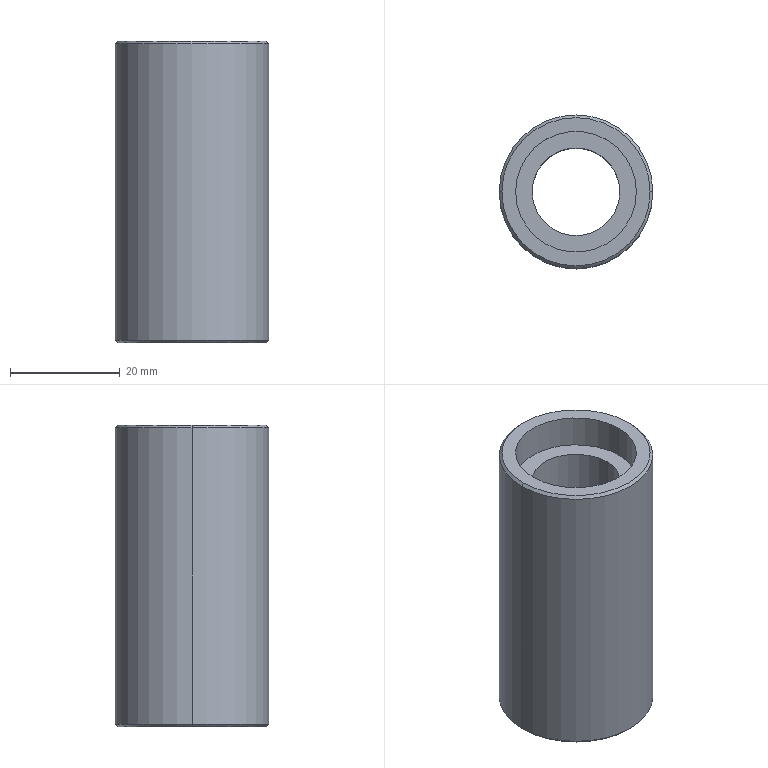Part | STEP file | 2017 Hold-down shaft | 1 solid | 16 faces | box 28 x 28 x 55 mm | volume 20637 mm3 | cylinder 8 | cone 4 | plane 4 | commonest cylinder face diameters 22 x4 16 x2 28 x2
STEP:
#1=CARTESIAN_POINT('',(0.,0.,0.));
#2=DIRECTION('',(0.,0.,1.));
#3=DIRECTION('',(1.,0.,0.));
#4=AXIS2_PLACEMENT_3D('',#1,#2,#3);
#5=CARTESIAN_POINT('',(-11.,0.,6.));
#6=VERTEX_POINT('',#5);
#7=CARTESIAN_POINT('',(-11.,0.,0.));
#8=VERTEX_POINT('',#7);
#9=CARTESIAN_POINT('',(-11.,0.,6.));
#10=DIRECTION('',(0.,0.,-1.));
#11=VECTOR('',#10,1.);
#12=LINE('',#9,#11);
#13=CARTESIAN_POINT('',(0.,0.,6.));
#14=DIRECTION('',(0.,0.,-1.));
#15=DIRECTION('',(-1.,0.,0.));
#16=AXIS2_PLACEMENT_3D('',#13,#14,#15);
#17=CYLINDRICAL_SURFACE('',#16,11.);
#18=CARTESIAN_POINT('',(6.283,0.));
#19=DIRECTION('',(0.,1.));
#20=VECTOR('',#19,1.);
#21=LINE('',#18,#20);
#22=(GEOMETRIC_REPRESENTATION_CONTEXT(2)PARAMETRIC_REPRESENTATION_CONTEXT()REPRESENTATION_CONTEXT('',''));
#23=DEFINITIONAL_REPRESENTATION('',(#21),#22);
#24=PCURVE('',#17,#23);
#25=CARTESIAN_POINT('',(0.,0.,6.));
#26=DIRECTION('',(0.,0.,-1.));
#27=DIRECTION('',(-1.,0.,0.));
#28=AXIS2_PLACEMENT_3D('',#25,#26,#27);
#29=CYLINDRICAL_SURFACE('',#28,11.);
#30=CARTESIAN_POINT('',(0.,0.));
#31=DIRECTION('',(0.,1.));
#32=VECTOR('',#31,1.);
#33=LINE('',#30,#32);
#34=(GEOMETRIC_REPRESENTATION_CONTEXT(2)PARAMETRIC_REPRESENTATION_CONTEXT()REPRESENTATION_CONTEXT('',''));
#35=DEFINITIONAL_REPRESENTATION('',(#33),#34);
#36=PCURVE('',#29,#35);
#37=SURFACE_CURVE('',#12,(#24,#36),.PCURVE_S1.);
#38=EDGE_CURVE('',#6,#8,#37,.T.);
#39=ORIENTED_EDGE('',*,*,#38,.T.);
#40=CARTESIAN_POINT('',(11.,0.,0.));
#41=VERTEX_POINT('',#40);
#42=CARTESIAN_POINT('',(0.,0.,0.));
#43=DIRECTION('',(0.,0.,-1.));
#44=DIRECTION('',(-1.,0.,0.));
#45=AXIS2_PLACEMENT_3D('',#42,#43,#44);
#46=CIRCLE('',#45,11.);
#47=CARTESIAN_POINT('',(0.,6.));
#48=DIRECTION('',(1.,0.));
#49=VECTOR('',#48,1.);
#50=LINE('',#47,#49);
#51=(GEOMETRIC_REPRESENTATION_CONTEXT(2)PARAMETRIC_REPRESENTATION_CONTEXT()REPRESENTATION_CONTEXT('',''));
#52=DEFINITIONAL_REPRESENTATION('',(#50),#51);
#53=PCURVE('',#17,#52);
#54=CARTESIAN_POINT('',(0.,0.,0.));
#55=DIRECTION('',(0.,0.,1.));
#56=DIRECTION('',(1.,0.,0.));
#57=AXIS2_PLACEMENT_3D('',#54,#55,#56);
#58=PLANE('',#57);
#59=CARTESIAN_POINT('',(-11.,0.));
#60=CARTESIAN_POINT('',(-11.,19.053));
#61=CARTESIAN_POINT('',(5.5,9.526));
#62=CARTESIAN_POINT('',(22.,0.));
#63=CARTESIAN_POINT('',(5.5,-9.526));
#64=CARTESIAN_POINT('',(-11.,-19.053));
#65=CARTESIAN_POINT('',(-11.,0.));
#66=(BOUNDED_CURVE()B_SPLINE_CURVE(2,(#59,#60,#61,#62,#63,#64,#65),.UNSPECIFIED.,.T.,.F.)B_SPLINE_CURVE_WITH_KNOTS((1,2,2,2,2,1),(-2.094,0.,2.094,4.189,6.283,8.378),.UNSPECIFIED.)CURVE()GEOMETRIC_REPRESENTATION_ITEM()RATIONAL_B_SPLINE_CURVE((1.,0.5,1.,0.5,1.,0.5,1.))REPRESENTATION_ITEM(''));
#67=(GEOMETRIC_REPRESENTATION_CONTEXT(2)PARAMETRIC_REPRESENTATION_CONTEXT()REPRESENTATION_CONTEXT('',''));
#68=DEFINITIONAL_REPRESENTATION('',(#66),#67);
#69=PCURVE('',#58,#68);
#70=SURFACE_CURVE('',#46,(#53,#69),.PCURVE_S1.);
#71=EDGE_CURVE('',#41,#8,#70,.T.);
#72=ORIENTED_EDGE('',*,*,#71,.F.);
#73=CARTESIAN_POINT('',(11.,0.,6.));
#74=VERTEX_POINT('',#73);
#75=CARTESIAN_POINT('',(11.,0.,6.));
#76=DIRECTION('',(0.,0.,-1.));
#77=VECTOR('',#76,1.);
#78=LINE('',#75,#77);
#79=CARTESIAN_POINT('',(3.142,0.));
#80=DIRECTION('',(0.,1.));
#81=VECTOR('',#80,1.);
#82=LINE('',#79,#81);
#83=(GEOMETRIC_REPRESENTATION_CONTEXT(2)PARAMETRIC_REPRESENTATION_CONTEXT()REPRESENTATION_CONTEXT('',''));
#84=DEFINITIONAL_REPRESENTATION('',(#82),#83);
#85=PCURVE('',#17,#84);
#86=CARTESIAN_POINT('',(3.142,0.));
#87=DIRECTION('',(0.,1.));
#88=VECTOR('',#87,1.);
#89=LINE('',#86,#88);
#90=(GEOMETRIC_REPRESENTATION_CONTEXT(2)PARAMETRIC_REPRESENTATION_CONTEXT()REPRESENTATION_CONTEXT('',''));
#91=DEFINITIONAL_REPRESENTATION('',(#89),#90);
#92=PCURVE('',#29,#91);
#93=SURFACE_CURVE('',#78,(#85,#92),.PCURVE_S1.);
#94=EDGE_CURVE('',#74,#41,#93,.T.);
#95=ORIENTED_EDGE('',*,*,#94,.F.);
#96=CARTESIAN_POINT('',(0.,0.,6.));
#97=DIRECTION('',(0.,0.,-1.));
#98=DIRECTION('',(-1.,0.,0.));
#99=AXIS2_PLACEMENT_3D('',#96,#97,#98);
#100=CIRCLE('',#99,11.);
#101=CARTESIAN_POINT('',(0.,0.));
#102=DIRECTION('',(1.,0.));
#103=VECTOR('',#102,1.);
#104=LINE('',#101,#103);
#105=(GEOMETRIC_REPRESENTATION_CONTEXT(2)PARAMETRIC_REPRESENTATION_CONTEXT()REPRESENTATION_CONTEXT('',''));
#106=DEFINITIONAL_REPRESENTATION('',(#104),#105);
#107=PCURVE('',#17,#106);
#108=CARTESIAN_POINT('',(0.,0.,6.));
#109=DIRECTION('',(0.,0.,-1.));
#110=DIRECTION('',(-1.,0.,0.));
#111=AXIS2_PLACEMENT_3D('',#108,#109,#110);
#112=PLANE('',#111);
#113=CARTESIAN_POINT('',(0.,0.));
#114=DIRECTION('',(1.,0.));
#115=AXIS2_PLACEMENT_2D('',#113,#114);
#116=CIRCLE('',#115,11.);
#117=(GEOMETRIC_REPRESENTATION_CONTEXT(2)PARAMETRIC_REPRESENTATION_CONTEXT()REPRESENTATION_CONTEXT('',''));
#118=DEFINITIONAL_REPRESENTATION('',(#116),#117);
#119=PCURVE('',#112,#118);
#120=SURFACE_CURVE('',#100,(#107,#119),.PCURVE_S1.);
#121=EDGE_CURVE('',#74,#6,#120,.T.);
#122=ORIENTED_EDGE('',*,*,#121,.T.);
#123=EDGE_LOOP('',(#39,#72,#95,#122));
#124=FACE_BOUND('',#123,.F.);
#125=ADVANCED_FACE('',(#124),#17,.F.);
#126=CARTESIAN_POINT('',(11.,0.,49.));
#127=VERTEX_POINT('',#126);
#128=CARTESIAN_POINT('',(11.,0.,55.));
#129=VERTEX_POINT('',#128);
#130=CARTESIAN_POINT('',(11.,0.,49.));
#131=DIRECTION('',(0.,0.,1.));
#132=VECTOR('',#131,1.);
#133=LINE('',#130,#132);
#134=CARTESIAN_POINT('',(0.,0.,49.));
#135=DIRECTION('',(0.,0.,1.));
#136=DIRECTION('',(1.,0.,0.));
#137=AXIS2_PLACEMENT_3D('',#134,#135,#136);
#138=CYLINDRICAL_SURFACE('',#137,11.);
#139=CARTESIAN_POINT('',(6.283,0.));
#140=DIRECTION('',(0.,1.));
#141=VECTOR('',#140,1.);
#142=LINE('',#139,#141);
#143=(GEOMETRIC_REPRESENTATION_CONTEXT(2)PARAMETRIC_REPRESENTATION_CONTEXT()REPRESENTATION_CONTEXT('',''));
#144=DEFINITIONAL_REPRESENTATION('',(#142),#143);
#145=PCURVE('',#138,#144);
#146=CARTESIAN_POINT('',(0.,0.,49.));
#147=DIRECTION('',(0.,0.,1.));
#148=DIRECTION('',(1.,0.,0.));
#149=AXIS2_PLACEMENT_3D('',#146,#147,#148);
#150=CYLINDRICAL_SURFACE('',#149,11.);
#151=CARTESIAN_POINT('',(0.,0.));
#152=DIRECTION('',(0.,1.));
#153=VECTOR('',#152,1.);
#154=LINE('',#151,#153);
#155=(GEOMETRIC_REPRESENTATION_CONTEXT(2)PARAMETRIC_REPRESENTATION_CONTEXT()REPRESENTATION_CONTEXT('',''));
#156=DEFINITIONAL_REPRESENTATION('',(#154),#155);
#157=PCURVE('',#150,#156);
#158=SURFACE_CURVE('',#133,(#145,#157),.PCURVE_S1.);
#159=EDGE_CURVE('',#127,#129,#158,.T.);
#160=ORIENTED_EDGE('',*,*,#159,.T.);
#161=CARTESIAN_POINT('',(-11.,0.,55.));
#162=VERTEX_POINT('',#161);
#163=CARTESIAN_POINT('',(0.,0.,55.));
#164=DIRECTION('',(0.,0.,1.));
#165=DIRECTION('',(1.,0.,0.));
#166=AXIS2_PLACEMENT_3D('',#163,#164,#165);
#167=CIRCLE('',#166,11.);
#168=CARTESIAN_POINT('',(0.,6.));
#169=DIRECTION('',(1.,0.));
#170=VECTOR('',#169,1.);
#171=LINE('',#168,#170);
#172=(GEOMETRIC_REPRESENTATION_CONTEXT(2)PARAMETRIC_REPRESENTATION_CONTEXT()REPRESENTATION_CONTEXT('',''));
#173=DEFINITIONAL_REPRESENTATION('',(#171),#172);
#174=PCURVE('',#138,#173);
#175=CARTESIAN_POINT('',(0.,0.,55.));
#176=DIRECTION('',(0.,0.,1.));
#177=DIRECTION('',(1.,0.,0.));
#178=AXIS2_PLACEMENT_3D('',#175,#176,#177);
#179=PLANE('',#178);
#180=CARTESIAN_POINT('',(0.,0.));
#181=DIRECTION('',(1.,0.));
#182=AXIS2_PLACEMENT_2D('',#180,#181);
#183=CIRCLE('',#182,11.);
#184=(GEOMETRIC_REPRESENTATION_CONTEXT(2)PARAMETRIC_REPRESENTATION_CONTEXT()REPRESENTATION_CONTEXT('',''));
#185=DEFINITIONAL_REPRESENTATION('',(#183),#184);
#186=PCURVE('',#179,#185);
#187=SURFACE_CURVE('',#167,(#174,#186),.PCURVE_S1.);
#188=EDGE_CURVE('',#162,#129,#187,.T.);
#189=ORIENTED_EDGE('',*,*,#188,.F.);
#190=CARTESIAN_POINT('',(-11.,0.,49.));
#191=VERTEX_POINT('',#190);
#192=CARTESIAN_POINT('',(-11.,0.,49.));
#193=DIRECTION('',(0.,0.,1.));
#194=VECTOR('',#193,1.);
#195=LINE('',#192,#194);
#196=CARTESIAN_POINT('',(3.142,0.));
#197=DIRECTION('',(0.,1.));
#198=VECTOR('',#197,1.);
#199=LINE('',#196,#198);
#200=(GEOMETRIC_REPRESENTATION_CONTEXT(2)PARAMETRIC_REPRESENTATION_CONTEXT()REPRESENTATION_CONTEXT('',''));
#201=DEFINITIONAL_REPRESENTATION('',(#199),#200);
#202=PCURVE('',#138,#201);
#203=CARTESIAN_POINT('',(3.142,0.));
#204=DIRECTION('',(0.,1.));
#205=VECTOR('',#204,1.);
#206=LINE('',#203,#205);
#207=(GEOMETRIC_REPRESENTATION_CONTEXT(2)PARAMETRIC_REPRESENTATION_CONTEXT()REPRESENTATION_CONTEXT('',''));
#208=DEFINITIONAL_REPRESENTATION('',(#206),#207);
#209=PCURVE('',#150,#208);
#210=SURFACE_CURVE('',#195,(#202,#209),.PCURVE_S1.);
#211=EDGE_CURVE('',#191,#162,#210,.T.);
#212=ORIENTED_EDGE('',*,*,#211,.F.);
#213=CARTESIAN_POINT('',(0.,0.,49.));
#214=DIRECTION('',(0.,0.,1.));
#215=DIRECTION('',(1.,0.,0.));
#216=AXIS2_PLACEMENT_3D('',#213,#214,#215);
#217=CIRCLE('',#216,11.);
#218=CARTESIAN_POINT('',(0.,0.));
#219=DIRECTION('',(1.,0.));
#220=VECTOR('',#219,1.);
#221=LINE('',#218,#220);
#222=(GEOMETRIC_REPRESENTATION_CONTEXT(2)PARAMETRIC_REPRESENTATION_CONTEXT()REPRESENTATION_CONTEXT('',''));
#223=DEFINITIONAL_REPRESENTATION('',(#221),#222);
#224=PCURVE('',#138,#223);
#225=CARTESIAN_POINT('',(0.,0.,49.));
#226=DIRECTION('',(0.,0.,1.));
#227=DIRECTION('',(1.,0.,0.));
#228=AXIS2_PLACEMENT_3D('',#225,#226,#227);
#229=PLANE('',#228);
#230=CARTESIAN_POINT('',(0.,0.));
#231=DIRECTION('',(1.,0.));
#232=AXIS2_PLACEMENT_2D('',#230,#231);
#233=CIRCLE('',#232,11.);
#234=(GEOMETRIC_REPRESENTATION_CONTEXT(2)PARAMETRIC_REPRESENTATION_CONTEXT()REPRESENTATION_CONTEXT('',''));
#235=DEFINITIONAL_REPRESENTATION('',(#233),#234);
#236=PCURVE('',#229,#235);
#237=SURFACE_CURVE('',#217,(#224,#236),.PCURVE_S1.);
#238=EDGE_CURVE('',#191,#127,#237,.T.);
#239=ORIENTED_EDGE('',*,*,#238,.T.);
#240=EDGE_LOOP('',(#160,#189,#212,#239));
#241=FACE_BOUND('',#240,.F.);
#242=ADVANCED_FACE('',(#241),#138,.F.);
#243=CARTESIAN_POINT('',(13.5,0.,55.));
#244=VERTEX_POINT('',#243);
#245=CARTESIAN_POINT('',(-13.5,0.,55.));
#246=VERTEX_POINT('',#245);
#247=CARTESIAN_POINT('',(0.,0.,55.));
#248=DIRECTION('',(0.,0.,1.));
#249=DIRECTION('',(1.,0.,0.));
#250=AXIS2_PLACEMENT_3D('',#247,#248,#249);
#251=CIRCLE('',#250,13.5);
#252=CARTESIAN_POINT('',(0.,0.,55.));
#253=DIRECTION('',(0.,0.,-1.));
#254=DIRECTION('',(-1.,0.,0.));
#255=AXIS2_PLACEMENT_3D('',#252,#253,#254);
#256=CONICAL_SURFACE('',#255,13.5,0.7854);
#257=CARTESIAN_POINT('',(3.142,0.));
#258=DIRECTION('',(-1.,0.));
#259=VECTOR('',#258,1.);
#260=LINE('',#257,#259);
#261=(GEOMETRIC_REPRESENTATION_CONTEXT(2)PARAMETRIC_REPRESENTATION_CONTEXT()REPRESENTATION_CONTEXT('',''));
#262=DEFINITIONAL_REPRESENTATION('',(#260),#261);
#263=PCURVE('',#256,#262);
#264=CARTESIAN_POINT('',(0.,0.));
#265=DIRECTION('',(1.,0.));
#266=AXIS2_PLACEMENT_2D('',#264,#265);
#267=CIRCLE('',#266,13.5);
#268=(GEOMETRIC_REPRESENTATION_CONTEXT(2)PARAMETRIC_REPRESENTATION_CONTEXT()REPRESENTATION_CONTEXT('',''));
#269=DEFINITIONAL_REPRESENTATION('',(#267),#268);
#270=PCURVE('',#179,#269);
#271=SURFACE_CURVE('',#251,(#263,#270),.PCURVE_S1.);
#272=EDGE_CURVE('',#244,#246,#271,.T.);
#273=ORIENTED_EDGE('',*,*,#272,.F.);
#274=CARTESIAN_POINT('',(14.,0.,54.5));
#275=VERTEX_POINT('',#274);
#276=CARTESIAN_POINT('',(13.5,0.,55.));
#277=DIRECTION('',(0.7071,0.,-0.7071));
#278=VECTOR('',#277,1.);
#279=LINE('',#276,#278);
#280=CARTESIAN_POINT('',(3.142,0.));
#281=DIRECTION('',(0.,1.));
#282=VECTOR('',#281,1.);
#283=LINE('',#280,#282);
#284=(GEOMETRIC_REPRESENTATION_CONTEXT(2)PARAMETRIC_REPRESENTATION_CONTEXT()REPRESENTATION_CONTEXT('',''));
#285=DEFINITIONAL_REPRESENTATION('',(#283),#284);
#286=PCURVE('',#256,#285);
#287=CARTESIAN_POINT('',(0.,0.,55.));
#288=DIRECTION('',(0.,0.,-1.));
#289=DIRECTION('',(-1.,0.,0.));
#290=AXIS2_PLACEMENT_3D('',#287,#288,#289);
#291=CONICAL_SURFACE('',#290,13.5,0.7854);
#292=CARTESIAN_POINT('',(3.142,0.));
#293=DIRECTION('',(0.,1.));
#294=VECTOR('',#293,1.);
#295=LINE('',#292,#294);
#296=(GEOMETRIC_REPRESENTATION_CONTEXT(2)PARAMETRIC_REPRESENTATION_CONTEXT()REPRESENTATION_CONTEXT('',''));
#297=DEFINITIONAL_REPRESENTATION('',(#295),#296);
#298=PCURVE('',#291,#297);
#299=SURFACE_CURVE('',#279,(#286,#298),.PCURVE_S1.);
#300=EDGE_CURVE('',#244,#275,#299,.T.);
#301=ORIENTED_EDGE('',*,*,#300,.T.);
#302=CARTESIAN_POINT('',(-14.,0.,54.5));
#303=VERTEX_POINT('',#302);
#304=CARTESIAN_POINT('',(0.,0.,54.5));
#305=DIRECTION('',(0.,0.,-1.));
#306=DIRECTION('',(1.,0.,0.));
#307=AXIS2_PLACEMENT_3D('',#304,#305,#306);
#308=CIRCLE('',#307,14.);
#309=CARTESIAN_POINT('',(-3.142,0.5));
#310=DIRECTION('',(1.,0.));
#311=VECTOR('',#310,1.);
#312=LINE('',#309,#311);
#313=(GEOMETRIC_REPRESENTATION_CONTEXT(2)PARAMETRIC_REPRESENTATION_CONTEXT()REPRESENTATION_CONTEXT('',''));
#314=DEFINITIONAL_REPRESENTATION('',(#312),#313);
#315=PCURVE('',#256,#314);
#316=CARTESIAN_POINT('',(0.,0.,55.));
#317=DIRECTION('',(0.,0.,-1.));
#318=DIRECTION('',(-1.,0.,0.));
#319=AXIS2_PLACEMENT_3D('',#316,#317,#318);
#320=CYLINDRICAL_SURFACE('',#319,14.);
#321=CARTESIAN_POINT('',(-3.142,0.5));
#322=DIRECTION('',(1.,0.));
#323=VECTOR('',#322,1.);
#324=LINE('',#321,#323);
#325=(GEOMETRIC_REPRESENTATION_CONTEXT(2)PARAMETRIC_REPRESENTATION_CONTEXT()REPRESENTATION_CONTEXT('',''));
#326=DEFINITIONAL_REPRESENTATION('',(#324),#325);
#327=PCURVE('',#320,#326);
#328=SURFACE_CURVE('',#308,(#315,#327),.PCURVE_S1.);
#329=EDGE_CURVE('',#303,#275,#328,.T.);
#330=ORIENTED_EDGE('',*,*,#329,.F.);
#331=CARTESIAN_POINT('',(-13.5,0.,55.));
#332=DIRECTION('',(-0.7071,0.,-0.7071));
#333=VECTOR('',#332,1.);
#334=LINE('',#331,#333);
#335=CARTESIAN_POINT('',(0.,0.));
#336=DIRECTION('',(0.,1.));
#337=VECTOR('',#336,1.);
#338=LINE('',#335,#337);
#339=(GEOMETRIC_REPRESENTATION_CONTEXT(2)PARAMETRIC_REPRESENTATION_CONTEXT()REPRESENTATION_CONTEXT('',''));
#340=DEFINITIONAL_REPRESENTATION('',(#338),#339);
#341=PCURVE('',#256,#340);
#342=CARTESIAN_POINT('',(6.283,0.));
#343=DIRECTION('',(0.,1.));
#344=VECTOR('',#343,1.);
#345=LINE('',#342,#344);
#346=(GEOMETRIC_REPRESENTATION_CONTEXT(2)PARAMETRIC_REPRESENTATION_CONTEXT()REPRESENTATION_CONTEXT('',''));
#347=DEFINITIONAL_REPRESENTATION('',(#345),#346);
#348=PCURVE('',#291,#347);
#349=SURFACE_CURVE('',#334,(#341,#348),.PCURVE_S1.);
#350=EDGE_CURVE('',#246,#303,#349,.T.);
#351=ORIENTED_EDGE('',*,*,#350,.F.);
#352=EDGE_LOOP('',(#273,#301,#330,#351));
#353=FACE_BOUND('',#352,.T.);
#354=ADVANCED_FACE('',(#353),#256,.T.);
#355=CARTESIAN_POINT('',(-13.5,0.,0.));
#356=VERTEX_POINT('',#355);
#357=CARTESIAN_POINT('',(13.5,0.,0.));
#358=VERTEX_POINT('',#357);
#359=CARTESIAN_POINT('',(0.,0.,0.));
#360=DIRECTION('',(0.,0.,-1.));
#361=DIRECTION('',(1.,0.,0.));
#362=AXIS2_PLACEMENT_3D('',#359,#360,#361);
#363=CIRCLE('',#362,13.5);
#364=CARTESIAN_POINT('',(0.,0.,0.5));
#365=DIRECTION('',(0.,0.,1.));
#366=DIRECTION('',(1.,0.,0.));
#367=AXIS2_PLACEMENT_3D('',#364,#365,#366);
#368=CONICAL_SURFACE('',#367,14.,0.7854);
#369=CARTESIAN_POINT('',(6.283,-0.5));
#370=DIRECTION('',(-1.,0.));
#371=VECTOR('',#370,1.);
#372=LINE('',#369,#371);
#373=(GEOMETRIC_REPRESENTATION_CONTEXT(2)PARAMETRIC_REPRESENTATION_CONTEXT()REPRESENTATION_CONTEXT('',''));
#374=DEFINITIONAL_REPRESENTATION('',(#372),#373);
#375=PCURVE('',#368,#374);
#376=CARTESIAN_POINT('',(13.5,0.));
#377=CARTESIAN_POINT('',(13.5,-23.383));
#378=CARTESIAN_POINT('',(-6.75,-11.691));
#379=CARTESIAN_POINT('',(-27.,0.));
#380=CARTESIAN_POINT('',(-6.75,11.691));
#381=CARTESIAN_POINT('',(13.5,23.383));
#382=CARTESIAN_POINT('',(13.5,0.));
#383=(BOUNDED_CURVE()B_SPLINE_CURVE(2,(#376,#377,#378,#379,#380,#381,#382),.UNSPECIFIED.,.T.,.F.)B_SPLINE_CURVE_WITH_KNOTS((1,2,2,2,2,1),(-2.094,0.,2.094,4.189,6.283,8.378),.UNSPECIFIED.)CURVE()GEOMETRIC_REPRESENTATION_ITEM()RATIONAL_B_SPLINE_CURVE((1.,0.5,1.,0.5,1.,0.5,1.))REPRESENTATION_ITEM(''));
#384=(GEOMETRIC_REPRESENTATION_CONTEXT(2)PARAMETRIC_REPRESENTATION_CONTEXT()REPRESENTATION_CONTEXT('',''));
#385=DEFINITIONAL_REPRESENTATION('',(#383),#384);
#386=PCURVE('',#58,#385);
#387=SURFACE_CURVE('',#363,(#375,#386),.PCURVE_S1.);
#388=EDGE_CURVE('',#356,#358,#387,.T.);
#389=ORIENTED_EDGE('',*,*,#388,.F.);
#390=CARTESIAN_POINT('',(-14.,0.,0.5));
#391=VERTEX_POINT('',#390);
#392=CARTESIAN_POINT('',(-14.,0.,0.5));
#393=DIRECTION('',(-0.7071,0.,0.7071));
#394=VECTOR('',#393,1.);
#395=LINE('',#392,#394);
#396=CARTESIAN_POINT('',(3.142,0.));
#397=DIRECTION('',(0.,1.));
#398=VECTOR('',#397,1.);
#399=LINE('',#396,#398);
#400=(GEOMETRIC_REPRESENTATION_CONTEXT(2)PARAMETRIC_REPRESENTATION_CONTEXT()REPRESENTATION_CONTEXT('',''));
#401=DEFINITIONAL_REPRESENTATION('',(#399),#400);
#402=PCURVE('',#368,#401);
#403=CARTESIAN_POINT('',(0.,0.,0.5));
#404=DIRECTION('',(0.,0.,1.));
#405=DIRECTION('',(1.,0.,0.));
#406=AXIS2_PLACEMENT_3D('',#403,#404,#405);
#407=CONICAL_SURFACE('',#406,14.,0.7854);
#408=CARTESIAN_POINT('',(3.142,0.));
#409=DIRECTION('',(0.,1.));
#410=VECTOR('',#409,1.);
#411=LINE('',#408,#410);
#412=(GEOMETRIC_REPRESENTATION_CONTEXT(2)PARAMETRIC_REPRESENTATION_CONTEXT()REPRESENTATION_CONTEXT('',''));
#413=DEFINITIONAL_REPRESENTATION('',(#411),#412);
#414=PCURVE('',#407,#413);
#415=SURFACE_CURVE('',#395,(#402,#414),.PCURVE_S1.);
#416=EDGE_CURVE('',#356,#391,#415,.T.);
#417=ORIENTED_EDGE('',*,*,#416,.T.);
#418=CARTESIAN_POINT('',(14.,0.,0.5));
#419=VERTEX_POINT('',#418);
#420=CARTESIAN_POINT('',(0.,0.,0.5));
#421=DIRECTION('',(0.,0.,1.));
#422=DIRECTION('',(1.,0.,0.));
#423=AXIS2_PLACEMENT_3D('',#420,#421,#422);
#424=CIRCLE('',#423,14.);
#425=CARTESIAN_POINT('',(0.,0.));
#426=DIRECTION('',(1.,0.));
#427=VECTOR('',#426,1.);
#428=LINE('',#425,#427);
#429=(GEOMETRIC_REPRESENTATION_CONTEXT(2)PARAMETRIC_REPRESENTATION_CONTEXT()REPRESENTATION_CONTEXT('',''));
#430=DEFINITIONAL_REPRESENTATION('',(#428),#429);
#431=PCURVE('',#368,#430);
#432=CARTESIAN_POINT('',(3.142,54.5));
#433=DIRECTION('',(-1.,0.));
#434=VECTOR('',#433,1.);
#435=LINE('',#432,#434);
#436=(GEOMETRIC_REPRESENTATION_CONTEXT(2)PARAMETRIC_REPRESENTATION_CONTEXT()REPRESENTATION_CONTEXT('',''));
#437=DEFINITIONAL_REPRESENTATION('',(#435),#436);
#438=PCURVE('',#320,#437);
#439=SURFACE_CURVE('',#424,(#431,#438),.PCURVE_S1.);
#440=EDGE_CURVE('',#419,#391,#439,.T.);
#441=ORIENTED_EDGE('',*,*,#440,.F.);
#442=CARTESIAN_POINT('',(14.,0.,0.5));
#443=DIRECTION('',(0.7071,0.,0.7071));
#444=VECTOR('',#443,1.);
#445=LINE('',#442,#444);
#446=CARTESIAN_POINT('',(0.,0.));
#447=DIRECTION('',(0.,1.));
#448=VECTOR('',#447,1.);
#449=LINE('',#446,#448);
#450=(GEOMETRIC_REPRESENTATION_CONTEXT(2)PARAMETRIC_REPRESENTATION_CONTEXT()REPRESENTATION_CONTEXT('',''));
#451=DEFINITIONAL_REPRESENTATION('',(#449),#450);
#452=PCURVE('',#368,#451);
#453=CARTESIAN_POINT('',(6.283,0.));
#454=DIRECTION('',(0.,1.));
#455=VECTOR('',#454,1.);
#456=LINE('',#453,#455);
#457=(GEOMETRIC_REPRESENTATION_CONTEXT(2)PARAMETRIC_REPRESENTATION_CONTEXT()REPRESENTATION_CONTEXT('',''));
#458=DEFINITIONAL_REPRESENTATION('',(#456),#457);
#459=PCURVE('',#407,#458);
#460=SURFACE_CURVE('',#445,(#452,#459),.PCURVE_S1.);
#461=EDGE_CURVE('',#358,#419,#460,.T.);
#462=ORIENTED_EDGE('',*,*,#461,.F.);
#463=EDGE_LOOP('',(#389,#417,#441,#462));
#464=FACE_BOUND('',#463,.T.);
#465=ADVANCED_FACE('',(#464),#368,.T.);
#466=ORIENTED_EDGE('',*,*,#329,.T.);
#467=CARTESIAN_POINT('',(14.,0.,55.));
#468=DIRECTION('',(0.,0.,-1.));
#469=VECTOR('',#468,1.);
#470=LINE('',#467,#469);
#471=CARTESIAN_POINT('',(3.142,0.));
#472=DIRECTION('',(0.,1.));
#473=VECTOR('',#472,1.);
#474=LINE('',#471,#473);
#475=(GEOMETRIC_REPRESENTATION_CONTEXT(2)PARAMETRIC_REPRESENTATION_CONTEXT()REPRESENTATION_CONTEXT('',''));
#476=DEFINITIONAL_REPRESENTATION('',(#474),#475);
#477=PCURVE('',#320,#476);
#478=CARTESIAN_POINT('',(0.,0.,55.));
#479=DIRECTION('',(0.,0.,-1.));
#480=DIRECTION('',(-1.,0.,0.));
#481=AXIS2_PLACEMENT_3D('',#478,#479,#480);
#482=CYLINDRICAL_SURFACE('',#481,14.);
#483=CARTESIAN_POINT('',(3.142,0.));
#484=DIRECTION('',(0.,1.));
#485=VECTOR('',#484,1.);
#486=LINE('',#483,#485);
#487=(GEOMETRIC_REPRESENTATION_CONTEXT(2)PARAMETRIC_REPRESENTATION_CONTEXT()REPRESENTATION_CONTEXT('',''));
#488=DEFINITIONAL_REPRESENTATION('',(#486),#487);
#489=PCURVE('',#482,#488);
#490=SURFACE_CURVE('',#470,(#477,#489),.PCURVE_S1.);
#491=EDGE_CURVE('',#275,#419,#490,.T.);
#492=ORIENTED_EDGE('',*,*,#491,.T.);
#493=ORIENTED_EDGE('',*,*,#440,.T.);
#494=CARTESIAN_POINT('',(-14.,0.,55.));
#495=DIRECTION('',(0.,0.,-1.));
#496=VECTOR('',#495,1.);
#497=LINE('',#494,#496);
#498=CARTESIAN_POINT('',(0.,0.));
#499=DIRECTION('',(0.,1.));
#500=VECTOR('',#499,1.);
#501=LINE('',#498,#500);
#502=(GEOMETRIC_REPRESENTATION_CONTEXT(2)PARAMETRIC_REPRESENTATION_CONTEXT()REPRESENTATION_CONTEXT('',''));
#503=DEFINITIONAL_REPRESENTATION('',(#501),#502);
#504=PCURVE('',#320,#503);
#505=CARTESIAN_POINT('',(6.283,0.));
#506=DIRECTION('',(0.,1.));
#507=VECTOR('',#506,1.);
#508=LINE('',#505,#507);
#509=(GEOMETRIC_REPRESENTATION_CONTEXT(2)PARAMETRIC_REPRESENTATION_CONTEXT()REPRESENTATION_CONTEXT('',''));
#510=DEFINITIONAL_REPRESENTATION('',(#508),#509);
#511=PCURVE('',#482,#510);
#512=SURFACE_CURVE('',#497,(#504,#511),.PCURVE_S1.);
#513=EDGE_CURVE('',#303,#391,#512,.T.);
#514=ORIENTED_EDGE('',*,*,#513,.F.);
#515=EDGE_LOOP('',(#466,#492,#493,#514));
#516=FACE_BOUND('',#515,.T.);
#517=ADVANCED_FACE('',(#516),#320,.T.);
#518=CARTESIAN_POINT('',(-8.,0.,49.));
#519=VERTEX_POINT('',#518);
#520=CARTESIAN_POINT('',(-8.,0.,6.));
#521=VERTEX_POINT('',#520);
#522=CARTESIAN_POINT('',(-8.,0.,55.));
#523=DIRECTION('',(0.,0.,-1.));
#524=VECTOR('',#523,1.);
#525=LINE('',#522,#524);
#526=CARTESIAN_POINT('',(0.,0.,55.));
#527=DIRECTION('',(0.,0.,-1.));
#528=DIRECTION('',(-1.,0.,0.));
#529=AXIS2_PLACEMENT_3D('',#526,#527,#528);
#530=CYLINDRICAL_SURFACE('',#529,8.);
#531=CARTESIAN_POINT('',(6.283,0.));
#532=DIRECTION('',(0.,1.));
#533=VECTOR('',#532,1.);
#534=LINE('',#531,#533);
#535=(GEOMETRIC_REPRESENTATION_CONTEXT(2)PARAMETRIC_REPRESENTATION_CONTEXT()REPRESENTATION_CONTEXT('',''));
#536=DEFINITIONAL_REPRESENTATION('',(#534),#535);
#537=PCURVE('',#530,#536);
#538=CARTESIAN_POINT('',(0.,0.,55.));
#539=DIRECTION('',(0.,0.,-1.));
#540=DIRECTION('',(-1.,0.,0.));
#541=AXIS2_PLACEMENT_3D('',#538,#539,#540);
#542=CYLINDRICAL_SURFACE('',#541,8.);
#543=CARTESIAN_POINT('',(0.,0.));
#544=DIRECTION('',(0.,1.));
#545=VECTOR('',#544,1.);
#546=LINE('',#543,#545);
#547=(GEOMETRIC_REPRESENTATION_CONTEXT(2)PARAMETRIC_REPRESENTATION_CONTEXT()REPRESENTATION_CONTEXT('',''));
#548=DEFINITIONAL_REPRESENTATION('',(#546),#547);
#549=PCURVE('',#542,#548);
#550=SURFACE_CURVE('',#525,(#537,#549),.PCURVE_S1.);
#551=EDGE_CURVE('',#519,#521,#550,.T.);
#552=ORIENTED_EDGE('',*,*,#551,.T.);
#553=CARTESIAN_POINT('',(8.,0.,6.));
#554=VERTEX_POINT('',#553);
#555=CARTESIAN_POINT('',(0.,0.,6.));
#556=DIRECTION('',(0.,0.,-1.));
#557=DIRECTION('',(-1.,0.,0.));
#558=AXIS2_PLACEMENT_3D('',#555,#556,#557);
#559=CIRCLE('',#558,8.);
#560=CARTESIAN_POINT('',(0.,49.));
#561=DIRECTION('',(1.,0.));
#562=VECTOR('',#561,1.);
#563=LINE('',#560,#562);
#564=(GEOMETRIC_REPRESENTATION_CONTEXT(2)PARAMETRIC_REPRESENTATION_CONTEXT()REPRESENTATION_CONTEXT('',''));
#565=DEFINITIONAL_REPRESENTATION('',(#563),#564);
#566=PCURVE('',#530,#565);
#567=CARTESIAN_POINT('',(0.,0.));
#568=DIRECTION('',(1.,0.));
#569=AXIS2_PLACEMENT_2D('',#567,#568);
#570=CIRCLE('',#569,8.);
#571=(GEOMETRIC_REPRESENTATION_CONTEXT(2)PARAMETRIC_REPRESENTATION_CONTEXT()REPRESENTATION_CONTEXT('',''));
#572=DEFINITIONAL_REPRESENTATION('',(#570),#571);
#573=PCURVE('',#112,#572);
#574=SURFACE_CURVE('',#559,(#566,#573),.PCURVE_S1.);
#575=EDGE_CURVE('',#554,#521,#574,.T.);
#576=ORIENTED_EDGE('',*,*,#575,.F.);
#577=CARTESIAN_POINT('',(8.,0.,49.));
#578=VERTEX_POINT('',#577);
#579=CARTESIAN_POINT('',(8.,0.,55.));
#580=DIRECTION('',(0.,0.,-1.));
#581=VECTOR('',#580,1.);
#582=LINE('',#579,#581);
#583=CARTESIAN_POINT('',(3.142,0.));
#584=DIRECTION('',(0.,1.));
#585=VECTOR('',#584,1.);
#586=LINE('',#583,#585);
#587=(GEOMETRIC_REPRESENTATION_CONTEXT(2)PARAMETRIC_REPRESENTATION_CONTEXT()REPRESENTATION_CONTEXT('',''));
#588=DEFINITIONAL_REPRESENTATION('',(#586),#587);
#589=PCURVE('',#530,#588);
#590=CARTESIAN_POINT('',(3.142,0.));
#591=DIRECTION('',(0.,1.));
#592=VECTOR('',#591,1.);
#593=LINE('',#590,#592);
#594=(GEOMETRIC_REPRESENTATION_CONTEXT(2)PARAMETRIC_REPRESENTATION_CONTEXT()REPRESENTATION_CONTEXT('',''));
#595=DEFINITIONAL_REPRESENTATION('',(#593),#594);
#596=PCURVE('',#542,#595);
#597=SURFACE_CURVE('',#582,(#589,#596),.PCURVE_S1.);
#598=EDGE_CURVE('',#578,#554,#597,.T.);
#599=ORIENTED_EDGE('',*,*,#598,.F.);
#600=CARTESIAN_POINT('',(0.,0.,49.));
#601=DIRECTION('',(0.,0.,1.));
#602=DIRECTION('',(1.,0.,0.));
#603=AXIS2_PLACEMENT_3D('',#600,#601,#602);
#604=CIRCLE('',#603,8.);
#605=CARTESIAN_POINT('',(9.425,6.));
#606=DIRECTION('',(-1.,0.));
#607=VECTOR('',#606,1.);
#608=LINE('',#605,#607);
#609=(GEOMETRIC_REPRESENTATION_CONTEXT(2)PARAMETRIC_REPRESENTATION_CONTEXT()REPRESENTATION_CONTEXT('',''));
#610=DEFINITIONAL_REPRESENTATION('',(#608),#609);
#611=PCURVE('',#530,#610);
#612=CARTESIAN_POINT('',(0.,0.));
#613=DIRECTION('',(1.,0.));
#614=AXIS2_PLACEMENT_2D('',#612,#613);
#615=CIRCLE('',#614,8.);
#616=(GEOMETRIC_REPRESENTATION_CONTEXT(2)PARAMETRIC_REPRESENTATION_CONTEXT()REPRESENTATION_CONTEXT('',''));
#617=DEFINITIONAL_REPRESENTATION('',(#615),#616);
#618=PCURVE('',#229,#617);
#619=SURFACE_CURVE('',#604,(#611,#618),.PCURVE_S1.);
#620=EDGE_CURVE('',#519,#578,#619,.T.);
#621=ORIENTED_EDGE('',*,*,#620,.F.);
#622=EDGE_LOOP('',(#552,#576,#599,#621));
#623=FACE_BOUND('',#622,.F.);
#624=ADVANCED_FACE('',(#623),#530,.F.);
#625=CARTESIAN_POINT('',(0.,0.,6.));
#626=DIRECTION('',(0.,0.,-1.));
#627=DIRECTION('',(-1.,0.,0.));
#628=AXIS2_PLACEMENT_3D('',#625,#626,#627);
#629=CIRCLE('',#628,8.);
#630=CARTESIAN_POINT('',(0.,49.));
#631=DIRECTION('',(1.,0.));
#632=VECTOR('',#631,1.);
#633=LINE('',#630,#632);
#634=(GEOMETRIC_REPRESENTATION_CONTEXT(2)PARAMETRIC_REPRESENTATION_CONTEXT()REPRESENTATION_CONTEXT('',''));
#635=DEFINITIONAL_REPRESENTATION('',(#633),#634);
#636=PCURVE('',#542,#635);
#637=CARTESIAN_POINT('',(0.,0.));
#638=DIRECTION('',(1.,0.));
#639=AXIS2_PLACEMENT_2D('',#637,#638);
#640=CIRCLE('',#639,8.);
#641=(GEOMETRIC_REPRESENTATION_CONTEXT(2)PARAMETRIC_REPRESENTATION_CONTEXT()REPRESENTATION_CONTEXT('',''));
#642=DEFINITIONAL_REPRESENTATION('',(#640),#641);
#643=PCURVE('',#112,#642);
#644=SURFACE_CURVE('',#629,(#636,#643),.PCURVE_S1.);
#645=EDGE_CURVE('',#521,#554,#644,.T.);
#646=ORIENTED_EDGE('',*,*,#645,.F.);
#647=ORIENTED_EDGE('',*,*,#551,.F.);
#648=CARTESIAN_POINT('',(0.,0.,49.));
#649=DIRECTION('',(0.,0.,1.));
#650=DIRECTION('',(1.,0.,0.));
#651=AXIS2_PLACEMENT_3D('',#648,#649,#650);
#652=CIRCLE('',#651,8.);
#653=CARTESIAN_POINT('',(3.142,6.));
#654=DIRECTION('',(-1.,0.));
#655=VECTOR('',#654,1.);
#656=LINE('',#653,#655);
#657=(GEOMETRIC_REPRESENTATION_CONTEXT(2)PARAMETRIC_REPRESENTATION_CONTEXT()REPRESENTATION_CONTEXT('',''));
#658=DEFINITIONAL_REPRESENTATION('',(#656),#657);
#659=PCURVE('',#542,#658);
#660=CARTESIAN_POINT('',(0.,0.));
#661=DIRECTION('',(1.,0.));
#662=AXIS2_PLACEMENT_2D('',#660,#661);
#663=CIRCLE('',#662,8.);
#664=(GEOMETRIC_REPRESENTATION_CONTEXT(2)PARAMETRIC_REPRESENTATION_CONTEXT()REPRESENTATION_CONTEXT('',''));
#665=DEFINITIONAL_REPRESENTATION('',(#663),#664);
#666=PCURVE('',#229,#665);
#667=SURFACE_CURVE('',#652,(#659,#666),.PCURVE_S1.);
#668=EDGE_CURVE('',#578,#519,#667,.T.);
#669=ORIENTED_EDGE('',*,*,#668,.F.);
#670=ORIENTED_EDGE('',*,*,#598,.T.);
#671=EDGE_LOOP('',(#646,#647,#669,#670));
#672=FACE_BOUND('',#671,.F.);
#673=ADVANCED_FACE('',(#672),#542,.F.);
#674=CARTESIAN_POINT('',(0.,0.,55.));
#675=DIRECTION('',(0.,0.,1.));
#676=DIRECTION('',(1.,0.,0.));
#677=AXIS2_PLACEMENT_3D('',#674,#675,#676);
#678=CIRCLE('',#677,11.);
#679=CARTESIAN_POINT('',(0.,0.));
#680=DIRECTION('',(1.,0.));
#681=AXIS2_PLACEMENT_2D('',#679,#680);
#682=CIRCLE('',#681,11.);
#683=(GEOMETRIC_REPRESENTATION_CONTEXT(2)PARAMETRIC_REPRESENTATION_CONTEXT()REPRESENTATION_CONTEXT('',''));
#684=DEFINITIONAL_REPRESENTATION('',(#682),#683);
#685=PCURVE('',#179,#684);
#686=CARTESIAN_POINT('',(0.,6.));
#687=DIRECTION('',(1.,0.));
#688=VECTOR('',#687,1.);
#689=LINE('',#686,#688);
#690=(GEOMETRIC_REPRESENTATION_CONTEXT(2)PARAMETRIC_REPRESENTATION_CONTEXT()REPRESENTATION_CONTEXT('',''));
#691=DEFINITIONAL_REPRESENTATION('',(#689),#690);
#692=PCURVE('',#150,#691);
#693=SURFACE_CURVE('',#678,(#685,#692),.PCURVE_S1.);
#694=EDGE_CURVE('',#129,#162,#693,.T.);
#695=ORIENTED_EDGE('',*,*,#694,.F.);
#696=ORIENTED_EDGE('',*,*,#188,.F.);
#697=EDGE_LOOP('',(#695,#696));
#698=FACE_BOUND('',#697,.T.);
#699=CARTESIAN_POINT('',(0.,0.,55.));
#700=DIRECTION('',(0.,0.,1.));
#701=DIRECTION('',(1.,0.,0.));
#702=AXIS2_PLACEMENT_3D('',#699,#700,#701);
#703=CIRCLE('',#702,13.5);
#704=CARTESIAN_POINT('',(0.,0.));
#705=DIRECTION('',(1.,0.));
#706=AXIS2_PLACEMENT_2D('',#704,#705);
#707=CIRCLE('',#706,13.5);
#708=(GEOMETRIC_REPRESENTATION_CONTEXT(2)PARAMETRIC_REPRESENTATION_CONTEXT()REPRESENTATION_CONTEXT('',''));
#709=DEFINITIONAL_REPRESENTATION('',(#707),#708);
#710=PCURVE('',#179,#709);
#711=CARTESIAN_POINT('',(9.425,0.));
#712=DIRECTION('',(-1.,0.));
#713=VECTOR('',#712,1.);
#714=LINE('',#711,#713);
#715=(GEOMETRIC_REPRESENTATION_CONTEXT(2)PARAMETRIC_REPRESENTATION_CONTEXT()REPRESENTATION_CONTEXT('',''));
#716=DEFINITIONAL_REPRESENTATION('',(#714),#715);
#717=PCURVE('',#291,#716);
#718=SURFACE_CURVE('',#703,(#710,#717),.PCURVE_S1.);
#719=EDGE_CURVE('',#246,#244,#718,.T.);
#720=ORIENTED_EDGE('',*,*,#719,.T.);
#721=ORIENTED_EDGE('',*,*,#272,.T.);
#722=EDGE_LOOP('',(#720,#721));
#723=FACE_BOUND('',#722,.T.);
#724=ADVANCED_FACE('',(#698,#723),#179,.T.);
#725=CARTESIAN_POINT('',(0.,0.,0.));
#726=DIRECTION('',(0.,0.,-1.));
#727=DIRECTION('',(-1.,0.,0.));
#728=AXIS2_PLACEMENT_3D('',#725,#726,#727);
#729=CIRCLE('',#728,11.);
#730=CARTESIAN_POINT('',(-11.,0.));
#731=CARTESIAN_POINT('',(-11.,19.053));
#732=CARTESIAN_POINT('',(5.5,9.526));
#733=CARTESIAN_POINT('',(22.,0.));
#734=CARTESIAN_POINT('',(5.5,-9.526));
#735=CARTESIAN_POINT('',(-11.,-19.053));
#736=CARTESIAN_POINT('',(-11.,0.));
#737=(BOUNDED_CURVE()B_SPLINE_CURVE(2,(#730,#731,#732,#733,#734,#735,#736),.UNSPECIFIED.,.T.,.F.)B_SPLINE_CURVE_WITH_KNOTS((1,2,2,2,2,1),(-2.094,0.,2.094,4.189,6.283,8.378),.UNSPECIFIED.)CURVE()GEOMETRIC_REPRESENTATION_ITEM()RATIONAL_B_SPLINE_CURVE((1.,0.5,1.,0.5,1.,0.5,1.))REPRESENTATION_ITEM(''));
#738=(GEOMETRIC_REPRESENTATION_CONTEXT(2)PARAMETRIC_REPRESENTATION_CONTEXT()REPRESENTATION_CONTEXT('',''));
#739=DEFINITIONAL_REPRESENTATION('',(#737),#738);
#740=PCURVE('',#58,#739);
#741=CARTESIAN_POINT('',(0.,6.));
#742=DIRECTION('',(1.,0.));
#743=VECTOR('',#742,1.);
#744=LINE('',#741,#743);
#745=(GEOMETRIC_REPRESENTATION_CONTEXT(2)PARAMETRIC_REPRESENTATION_CONTEXT()REPRESENTATION_CONTEXT('',''));
#746=DEFINITIONAL_REPRESENTATION('',(#744),#745);
#747=PCURVE('',#29,#746);
#748=SURFACE_CURVE('',#729,(#740,#747),.PCURVE_S1.);
#749=EDGE_CURVE('',#8,#41,#748,.T.);
#750=ORIENTED_EDGE('',*,*,#749,.F.);
#751=ORIENTED_EDGE('',*,*,#71,.F.);
#752=EDGE_LOOP('',(#750,#751));
#753=FACE_BOUND('',#752,.T.);
#754=CARTESIAN_POINT('',(0.,0.,0.));
#755=DIRECTION('',(0.,0.,-1.));
#756=DIRECTION('',(1.,0.,0.));
#757=AXIS2_PLACEMENT_3D('',#754,#755,#756);
#758=CIRCLE('',#757,13.5);
#759=CARTESIAN_POINT('',(13.5,0.));
#760=CARTESIAN_POINT('',(13.5,-23.383));
#761=CARTESIAN_POINT('',(-6.75,-11.691));
#762=CARTESIAN_POINT('',(-27.,0.));
#763=CARTESIAN_POINT('',(-6.75,11.691));
#764=CARTESIAN_POINT('',(13.5,23.383));
#765=CARTESIAN_POINT('',(13.5,0.));
#766=(BOUNDED_CURVE()B_SPLINE_CURVE(2,(#759,#760,#761,#762,#763,#764,#765),.UNSPECIFIED.,.T.,.F.)B_SPLINE_CURVE_WITH_KNOTS((1,2,2,2,2,1),(-2.094,0.,2.094,4.189,6.283,8.378),.UNSPECIFIED.)CURVE()GEOMETRIC_REPRESENTATION_ITEM()RATIONAL_B_SPLINE_CURVE((1.,0.5,1.,0.5,1.,0.5,1.))REPRESENTATION_ITEM(''));
#767=(GEOMETRIC_REPRESENTATION_CONTEXT(2)PARAMETRIC_REPRESENTATION_CONTEXT()REPRESENTATION_CONTEXT('',''));
#768=DEFINITIONAL_REPRESENTATION('',(#766),#767);
#769=PCURVE('',#58,#768);
#770=CARTESIAN_POINT('',(6.283,-0.5));
#771=DIRECTION('',(-1.,0.));
#772=VECTOR('',#771,1.);
#773=LINE('',#770,#772);
#774=(GEOMETRIC_REPRESENTATION_CONTEXT(2)PARAMETRIC_REPRESENTATION_CONTEXT()REPRESENTATION_CONTEXT('',''));
#775=DEFINITIONAL_REPRESENTATION('',(#773),#774);
#776=PCURVE('',#407,#775);
#777=SURFACE_CURVE('',#758,(#769,#776),.PCURVE_S1.);
#778=EDGE_CURVE('',#358,#356,#777,.T.);
#779=ORIENTED_EDGE('',*,*,#778,.T.);
#780=ORIENTED_EDGE('',*,*,#388,.T.);
#781=EDGE_LOOP('',(#779,#780));
#782=FACE_BOUND('',#781,.T.);
#783=ADVANCED_FACE('',(#753,#782),#58,.F.);
#784=ORIENTED_EDGE('',*,*,#491,.F.);
#785=CARTESIAN_POINT('',(0.,0.,54.5));
#786=DIRECTION('',(0.,0.,-1.));
#787=DIRECTION('',(1.,0.,0.));
#788=AXIS2_PLACEMENT_3D('',#785,#786,#787);
#789=CIRCLE('',#788,14.);
#790=CARTESIAN_POINT('',(3.142,0.5));
#791=DIRECTION('',(1.,0.));
#792=VECTOR('',#791,1.);
#793=LINE('',#790,#792);
#794=(GEOMETRIC_REPRESENTATION_CONTEXT(2)PARAMETRIC_REPRESENTATION_CONTEXT()REPRESENTATION_CONTEXT('',''));
#795=DEFINITIONAL_REPRESENTATION('',(#793),#794);
#796=PCURVE('',#482,#795);
#797=CARTESIAN_POINT('',(3.142,0.5));
#798=DIRECTION('',(1.,0.));
#799=VECTOR('',#798,1.);
#800=LINE('',#797,#799);
#801=(GEOMETRIC_REPRESENTATION_CONTEXT(2)PARAMETRIC_REPRESENTATION_CONTEXT()REPRESENTATION_CONTEXT('',''));
#802=DEFINITIONAL_REPRESENTATION('',(#800),#801);
#803=PCURVE('',#291,#802);
#804=SURFACE_CURVE('',#789,(#796,#803),.PCURVE_S1.);
#805=EDGE_CURVE('',#275,#303,#804,.T.);
#806=ORIENTED_EDGE('',*,*,#805,.T.);
#807=ORIENTED_EDGE('',*,*,#513,.T.);
#808=CARTESIAN_POINT('',(0.,0.,0.5));
#809=DIRECTION('',(0.,0.,1.));
#810=DIRECTION('',(1.,0.,0.));
#811=AXIS2_PLACEMENT_3D('',#808,#809,#810);
#812=CIRCLE('',#811,14.);
#813=CARTESIAN_POINT('',(9.425,54.5));
#814=DIRECTION('',(-1.,0.));
#815=VECTOR('',#814,1.);
#816=LINE('',#813,#815);
#817=(GEOMETRIC_REPRESENTATION_CONTEXT(2)PARAMETRIC_REPRESENTATION_CONTEXT()REPRESENTATION_CONTEXT('',''));
#818=DEFINITIONAL_REPRESENTATION('',(#816),#817);
#819=PCURVE('',#482,#818);
#820=CARTESIAN_POINT('',(0.,0.));
#821=DIRECTION('',(1.,0.));
#822=VECTOR('',#821,1.);
#823=LINE('',#820,#822);
#824=(GEOMETRIC_REPRESENTATION_CONTEXT(2)PARAMETRIC_REPRESENTATION_CONTEXT()REPRESENTATION_CONTEXT('',''));
#825=DEFINITIONAL_REPRESENTATION('',(#823),#824);
#826=PCURVE('',#407,#825);
#827=SURFACE_CURVE('',#812,(#819,#826),.PCURVE_S1.);
#828=EDGE_CURVE('',#391,#419,#827,.T.);
#829=ORIENTED_EDGE('',*,*,#828,.T.);
#830=EDGE_LOOP('',(#784,#806,#807,#829));
#831=FACE_BOUND('',#830,.T.);
#832=ADVANCED_FACE('',(#831),#482,.T.);
#833=ORIENTED_EDGE('',*,*,#416,.F.);
#834=ORIENTED_EDGE('',*,*,#778,.F.);
#835=ORIENTED_EDGE('',*,*,#461,.T.);
#836=ORIENTED_EDGE('',*,*,#828,.F.);
#837=EDGE_LOOP('',(#833,#834,#835,#836));
#838=FACE_BOUND('',#837,.T.);
#839=ADVANCED_FACE('',(#838),#407,.T.);
#840=ORIENTED_EDGE('',*,*,#300,.F.);
#841=ORIENTED_EDGE('',*,*,#719,.F.);
#842=ORIENTED_EDGE('',*,*,#350,.T.);
#843=ORIENTED_EDGE('',*,*,#805,.F.);
#844=EDGE_LOOP('',(#840,#841,#842,#843));
#845=FACE_BOUND('',#844,.T.);
#846=ADVANCED_FACE('',(#845),#291,.T.);
#847=ORIENTED_EDGE('',*,*,#694,.F.);
#848=ORIENTED_EDGE('',*,*,#159,.F.);
#849=CARTESIAN_POINT('',(0.,0.,49.));
#850=DIRECTION('',(0.,0.,1.));
#851=DIRECTION('',(1.,0.,0.));
#852=AXIS2_PLACEMENT_3D('',#849,#850,#851);
#853=CIRCLE('',#852,11.);
#854=CARTESIAN_POINT('',(0.,0.));
#855=DIRECTION('',(1.,0.));
#856=VECTOR('',#855,1.);
#857=LINE('',#854,#856);
#858=(GEOMETRIC_REPRESENTATION_CONTEXT(2)PARAMETRIC_REPRESENTATION_CONTEXT()REPRESENTATION_CONTEXT('',''));
#859=DEFINITIONAL_REPRESENTATION('',(#857),#858);
#860=PCURVE('',#150,#859);
#861=CARTESIAN_POINT('',(0.,0.));
#862=DIRECTION('',(1.,0.));
#863=AXIS2_PLACEMENT_2D('',#861,#862);
#864=CIRCLE('',#863,11.);
#865=(GEOMETRIC_REPRESENTATION_CONTEXT(2)PARAMETRIC_REPRESENTATION_CONTEXT()REPRESENTATION_CONTEXT('',''));
#866=DEFINITIONAL_REPRESENTATION('',(#864),#865);
#867=PCURVE('',#229,#866);
#868=SURFACE_CURVE('',#853,(#860,#867),.PCURVE_S1.);
#869=EDGE_CURVE('',#127,#191,#868,.T.);
#870=ORIENTED_EDGE('',*,*,#869,.T.);
#871=ORIENTED_EDGE('',*,*,#211,.T.);
#872=EDGE_LOOP('',(#847,#848,#870,#871));
#873=FACE_BOUND('',#872,.F.);
#874=ADVANCED_FACE('',(#873),#150,.F.);
#875=ORIENTED_EDGE('',*,*,#620,.F.);
#876=ORIENTED_EDGE('',*,*,#668,.F.);
#877=EDGE_LOOP('',(#875,#876));
#878=FACE_BOUND('',#877,.T.);
#879=ORIENTED_EDGE('',*,*,#869,.T.);
#880=ORIENTED_EDGE('',*,*,#238,.T.);
#881=EDGE_LOOP('',(#879,#880));
#882=FACE_BOUND('',#881,.T.);
#883=ADVANCED_FACE('',(#878,#882),#229,.T.);
#884=ORIENTED_EDGE('',*,*,#749,.F.);
#885=ORIENTED_EDGE('',*,*,#38,.F.);
#886=CARTESIAN_POINT('',(0.,0.,6.));
#887=DIRECTION('',(0.,0.,-1.));
#888=DIRECTION('',(-1.,0.,0.));
#889=AXIS2_PLACEMENT_3D('',#886,#887,#888);
#890=CIRCLE('',#889,11.);
#891=CARTESIAN_POINT('',(0.,0.));
#892=DIRECTION('',(1.,0.));
#893=VECTOR('',#892,1.);
#894=LINE('',#891,#893);
#895=(GEOMETRIC_REPRESENTATION_CONTEXT(2)PARAMETRIC_REPRESENTATION_CONTEXT()REPRESENTATION_CONTEXT('',''));
#896=DEFINITIONAL_REPRESENTATION('',(#894),#895);
#897=PCURVE('',#29,#896);
#898=CARTESIAN_POINT('',(0.,0.));
#899=DIRECTION('',(1.,0.));
#900=AXIS2_PLACEMENT_2D('',#898,#899);
#901=CIRCLE('',#900,11.);
#902=(GEOMETRIC_REPRESENTATION_CONTEXT(2)PARAMETRIC_REPRESENTATION_CONTEXT()REPRESENTATION_CONTEXT('',''));
#903=DEFINITIONAL_REPRESENTATION('',(#901),#902);
#904=PCURVE('',#112,#903);
#905=SURFACE_CURVE('',#890,(#897,#904),.PCURVE_S1.);
#906=EDGE_CURVE('',#6,#74,#905,.T.);
#907=ORIENTED_EDGE('',*,*,#906,.T.);
#908=ORIENTED_EDGE('',*,*,#94,.T.);
#909=EDGE_LOOP('',(#884,#885,#907,#908));
#910=FACE_BOUND('',#909,.F.);
#911=ADVANCED_FACE('',(#910),#29,.F.);
#912=ORIENTED_EDGE('',*,*,#645,.F.);
#913=ORIENTED_EDGE('',*,*,#575,.F.);
#914=EDGE_LOOP('',(#912,#913));
#915=FACE_BOUND('',#914,.T.);
#916=ORIENTED_EDGE('',*,*,#906,.T.);
#917=ORIENTED_EDGE('',*,*,#121,.T.);
#918=EDGE_LOOP('',(#916,#917));
#919=FACE_BOUND('',#918,.T.);
#920=ADVANCED_FACE('',(#915,#919),#112,.T.);
#921=CLOSED_SHELL('',(#125,#242,#354,#465,#517,#624,#673,#724,#783,#832,#839,#846,#874,#883,#911,#920));
#922=MANIFOLD_SOLID_BREP('',#921);
#923=(LENGTH_UNIT()NAMED_UNIT(*)SI_UNIT(.MILLI.,.METRE.));
#924=UNCERTAINTY_MEASURE_WITH_UNIT(LENGTH_MEASURE(0.0000001),#923,'','');
#925=(NAMED_UNIT(*)PLANE_ANGLE_UNIT()SI_UNIT($,.RADIAN.));
#926=(NAMED_UNIT(*)SI_UNIT($,.STERADIAN.)SOLID_ANGLE_UNIT());
#927=(GEOMETRIC_REPRESENTATION_CONTEXT(3)GLOBAL_UNCERTAINTY_ASSIGNED_CONTEXT((#924))GLOBAL_UNIT_ASSIGNED_CONTEXT((#923,#925,#926))REPRESENTATION_CONTEXT('',''));
#928=ADVANCED_BREP_SHAPE_REPRESENTATION('',(#4,#922),#927);